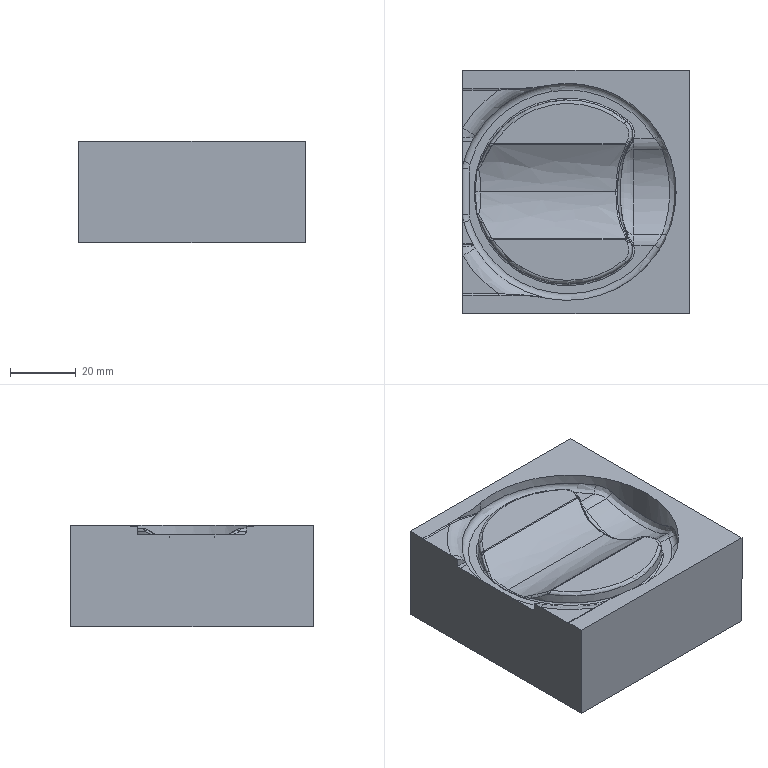NC program | NX | posted with a generic post | part box 69 x 74 x 31.001 mm
Lines 1117 to 2149 of 31411:
(CAVITY_MILL_COPY , TOOL : D4)
N2226 M6
N2228 G54
N2230 G17 G0 G90 X12.673 Y10.046 S3000 M3
N2232 G43 Z10.005 H0
N2234 Z-0.1
N2236 G94 G1 Z-0.3 F2500.
N2238 G3 X14.068 Y7.916 R3.
N2240 X14.297 Y7.776 R34.167
N2242 G1 X14.533 Y7.757
N2244 G3 X16.94 Y8.666 R3.
N2246 G1 Z-0.1
N2248 G0 Z0.305
N2250 X13.649 Y9.969
N2252 Z-0.25
N2254 G1 Z-0.45
N2256 G3 X15.101 Y7.876 R3.
N2258 X15.295 Y7.764 R33.672
N2260 G1 X15.409 Y7.743
N2262 X15.577 Y7.727
N2264 G3 X18.022 Y8.642 R3.
N2266 G1 Z-0.25
N2268 G0 Z0.
N2270 X14.426 Y9.899
N2272 Z-0.4
N2274 G1 Z-0.6
N2276 G3 X15.924 Y7.837 R3.
N2278 X16.12 Y7.73 R33.301
N2280 G1 X16.391 Y7.701
N2282 G3 X18.87 Y8.607 R3.
N2284 G1 Z-0.4
N2286 G0 Z-0.15
N2288 X15.106 Y9.829
N2290 Z-0.55
N2292 G1 Z-0.75
N2294 G3 X16.645 Y7.796 R3.
N2296 X16.893 Y7.667 R32.995
N2298 G2 X17.146 Y7.663 R52.17
N2300 G3 X19.356 Y8.582 R3.
N2302 G1 Z-0.55
N2304 G0 Z-0.3
N2306 X15.696 Y9.761
N2308 Z-0.7
N2310 G1 Z-0.9
N2312 G3 X17.27 Y7.755 R3.
N2314 X17.466 Y7.657 R32.745
N2316 G1 X17.665 Y7.652
N2318 G3 X19.884 Y8.549 R3.
N2320 G1 Z-0.7
N2322 G0 Z-0.45
N2324 X56.115 Y21.542
N2326 Z-0.843
N2328 G1 Z-1.043
N2330 G2 X55.66 Y20.526 R3.
N2332 X55.17 Y19.845 R28.83
N2334 G3 X55.097 Y20.583 R8.748
N2336 G2 X52.634 Y22.024 R4.06
N2338 X50.826 Y14.231 R6.748
N2340 X7.028 Y21.211 R29.544
N2342 X6.896 Y23.518 R2.382
N2344 G3 X7.155 Y25.291 R3.
N2346 G1 Z-0.843
N2348 G0 Z-0.6
N2350 X1.561 Y23.669
N2352 Z-0.843
N2354 G1 Z-1.043
N2356 G3 X2.694 Y22.308 R3.
N2358 G2 X3.485 Y21.41 R2.232
N2360 G1 X3.62 Y21.132
N2362 X4.229 Y20.072
N2364 X4.307 Y19.966
N2366 G3 X18.032 Y7.641 R32.512
N2368 G2 X26.165 Y6.727 R52.17
N2370 G3 X58.978 Y22.077 R30.83
N2372 X59.144 Y24.629 R3.
N2374 G1 Z-0.843
N2376 G0 Z-0.6
N2378 X56.27 Y21.786
N2380 Z-0.986
N2382 G1 Z-1.186
N2384 G2 X55.824 Y20.765 R3.
N2386 X55.358 Y20.101 R28.83
N2388 G3 X55.255 Y20.817 R9.856
N2390 G2 X52.692 Y22.346 R4.06
N2392 X53.392 Y19.644 R7.856
N2394 X50.952 Y14.079 R6.963
N2396 X6.729 Y21.317 R29.742
N2398 X6.627 Y23.748 R2.478
N2400 G3 X6.924 Y25.53 R3.
N2402 G1 Z-0.986
N2404 G0 Z-0.743
N2406 X1.486 Y23.67
N2408 Z-0.986
N2410 G1 Z-1.186
N2412 G3 X2.739 Y22.408 R3.
N2414 G2 X3.648 Y21.518 R2.244
N2416 G1 X4.372 Y20.219
N2418 X4.399 Y20.195
N2420 G3 X18.542 Y7.621 R32.314
N2422 G2 X26.165 Y6.727 R52.17
N2424 G3 X59.126 Y22.349 R30.83
N2426 X59.267 Y24.902 R3.
N2428 G1 Z-0.986
N2430 G0 Z-0.743
N2432 X56.359 Y21.93
N2434 Z-1.129
N2436 G1 Z-1.329
N2438 G2 X55.92 Y20.907 R3.
N2440 X55.474 Y20.262 R28.83
N2442 G3 X55.372 Y20.952 R8.855
N2444 G2 X52.734 Y22.527 R4.06
N2446 X52.97 Y22.01 R11.963
N2448 X51.542 Y14.485 R6.855
N2450 G1 X51.151 Y14.09
N2452 X51.036 Y13.977
N2454 G2 X6.622 Y21.239 R29.873
N2456 X6.418 Y23.934 R2.801
N2458 G3 X6.634 Y25.748 R3.
N2460 G1 Z-1.129
N2462 G0 Z-0.886
N2464 X1.458 Y23.67
N2466 Z-1.129
N2468 G1 Z-1.329
N2470 G3 X2.807 Y22.478 R3.
N2472 G2 X3.889 Y21.443 R2.217
N2474 G1 X4.044 Y21.132
N2476 X4.553 Y20.289
N2478 G3 X19.033 Y7.598 R32.134
N2480 G2 X26.165 Y6.727 R52.17
N2482 G3 X59.213 Y22.51 R30.83
N2484 X59.338 Y25.064 R3.
N2486 G1 Z-1.129
N2488 G0 Z-0.886
N2490 X56.416 Y22.021
N2492 Z-1.271
N2494 G1 Z-1.471
N2496 G2 X55.98 Y20.996 R3.
N2498 X55.558 Y20.382 R28.83
N2500 G3 X55.456 Y21.036 R8.975
N2502 G2 X52.828 Y22.553 R4.06
N2504 G1 X52.907 Y22.394
N2506 G2 X52.371 Y15.334 R6.975
N2508 G1 X52.354 Y15.309
N2510 G2 X51.095 Y13.905 R7.465
N2512 X6.471 Y21.307 R29.967
N2514 X6.266 Y24.16 R2.99
N2516 G3 X6.48 Y25.976 R3.
N2518 G1 Z-1.271
N2520 G0 Z-1.029
N2522 X1.227 Y23.67
N2524 Z-1.271
N2526 G1 Z-1.471
N2528 G3 X2.752 Y22.565 R3.
N2530 G2 X3.966 Y21.628 R2.24
N2532 G1 X4.659 Y20.398
N2534 X4.693 Y20.374
N2536 G3 X19.511 Y7.571 R31.97
N2538 G2 X26.165 Y6.727 R52.17
N2540 G3 X59.267 Y22.612 R30.83
N2542 X59.382 Y25.166 R3.
N2544 G1 Z-1.271
N2546 G0 Z-1.029
N2548 X56.469 Y22.109
N2550 Z-1.414
N2552 G1 Z-1.614
N2554 G2 X56.038 Y21.083 R3.
N2556 X55.618 Y20.466 R28.83
N2558 G3 X55.51 Y21.121 R9.082
N2560 G2 X52.85 Y22.667 R4.06
N2562 G1 X52.875 Y22.619
N2564 G2 X51.363 Y14.071 R7.082
N2566 G1 X51.169 Y13.892
N2568 X51.137 Y13.855
N2570 G2 X6.35 Y21.379 R30.032
N2572 X5.996 Y24.107 R3.403
N2574 G1 X6.035 Y24.226
N2576 G3 X6.115 Y26.019 R3.
N2578 G1 Z-1.414
N2580 G0 Z-1.171
N2582 X1.232 Y23.67
N2584 Z-1.414
N2586 G1 Z-1.614
N2588 G3 X2.833 Y22.592 R3.
N2590 G2 X4.134 Y21.628 R2.222
N2592 G1 X4.706 Y20.636
N2594 X4.823 Y20.453
N2596 G3 X19.979 Y7.54 R31.819
N2598 G2 X26.165 Y6.727 R52.17
N2600 G3 X59.318 Y22.71 R30.83
N2602 X59.425 Y25.265 R3.
N2604 G1 Z-1.414
N2606 G0 Z-1.171
N2608 X56.494 Y22.15
N2610 Z-1.557
N2612 G1 Z-1.757
N2614 G2 X56.064 Y21.123 R3.
N2616 X55.655 Y20.52 R28.83
N2618 G3 X55.548 Y21.159 R9.113
N2620 G2 X52.897 Y22.672 R4.06
N2622 G1 X52.924 Y22.619
N2624 G2 X51.858 Y14.509 R7.113
N2626 G1 X51.164 Y13.822
N2628 G2 X6.252 Y21.458 R30.075
N2630 X5.731 Y23.798 R3.914
N2632 X5.845 Y24.343 R2.473
N2634 G3 X5.866 Y26.148 R3.
N2636 G1 Z-1.557
N2638 G0 Z-1.314
N2640 X1.143 Y23.67
N2642 Z-1.557
N2644 G1 Z-1.757
N2646 G3 X2.865 Y22.624 R3.
N2648 G2 X4.302 Y21.628 R2.234
N2650 G1 X4.872 Y20.636
N2652 X4.942 Y20.525
N2654 G3 X20.442 Y7.505 R31.679
N2656 G2 X26.165 Y6.727 R52.17
N2658 G3 X59.342 Y22.756 R30.83
N2660 X59.444 Y25.311 R3.
N2662 G1 Z-1.557
N2664 G0 Z-1.314
N2666 X56.503 Y22.164
N2668 Z-1.7
N2670 G1 Z-1.9
N2672 G2 X56.073 Y21.136 R3.
N2674 X55.676 Y20.549 R28.83
N2676 G3 X55.57 Y21.17 R9.175
N2678 G2 X52.954 Y22.623 R4.06
N2680 G1 X52.984 Y22.563
N2682 G2 X51.385 Y13.991 R7.175
N2684 G1 X51.363 Y13.982
N2686 X51.193 Y13.838
N2688 X51.179 Y13.804
N2690 G2 X6.174 Y21.544 R30.097
N2692 X5.609 Y24.134 R4.083
N2694 X5.686 Y24.517 R2.426
N2696 G3 X5.637 Y26.315 R3.
N2698 G1 Z-1.7
N2700 G0 Z-1.457
N2702 X0.932 Y23.67
N2704 Z-1.7
N2706 G1 Z-1.9
N2708 G3 X2.842 Y22.654 R3.
N2710 G2 X4.448 Y21.628 R2.194
N2712 G1 X5.02 Y20.636
N2714 X5.052 Y20.593
N2716 G3 X20.905 Y7.466 R31.55
N2718 G2 X26.165 Y6.727 R52.17
N2720 G3 X59.35 Y22.771 R30.83
N2722 X59.451 Y25.326 R3.
N2724 G1 Z-1.7
N2726 G0 Z-1.457
N2728 X56.511 Y22.177
N2730 Z-1.843
N2732 G1 Z-2.043
N2734 G2 X56.082 Y21.15 R3.
N2736 X55.693 Y20.575 R28.83
N2738 G3 X55.588 Y21.182 R9.162
N2740 G2 X52.975 Y22.618 R4.06
N2742 X51.402 Y13.991 R7.162
N2744 G1 X51.363 Y13.969
N2746 X51.202 Y13.832
N2748 X51.189 Y13.802
N2750 G2 X6.041 Y21.753 R30.106
N2752 X5.439 Y24.142 R4.341
N2754 X5.518 Y24.669 R2.475
N2756 G3 X5.429 Y26.472 R3.
N2758 G1 Z-1.843
N2760 G0 Z-1.6
N2762 X0.586 Y23.707
N2764 Z-1.843
N2766 G1 Z-2.043
N2768 G3 X2.705 Y22.694 R3.
N2770 G1 X2.821 Y22.689
N2772 G2 X4.583 Y21.628 R2.17
N2774 G1 X5.155 Y20.655
N2776 G3 X21.371 Y7.422 R31.43
N2778 G2 X26.165 Y6.727 R52.17
N2780 G3 X59.358 Y22.786 R30.83
N2782 X59.457 Y25.341 R3.
N2784 G1 Z-1.843
N2786 G0 Z-1.6
N2788 X56.524 Y22.199
N2790 Z-1.986
N2792 G1 Z-2.186
N2794 G2 X56.096 Y21.171 R3.
N2796 X55.702 Y20.587 R28.83
N2798 G3 X55.594 Y21.204 R9.177
N2800 G2 X52.961 Y22.669 R4.06
N2802 X51.2 Y13.801 R7.177
N2804 X5.881 Y22.013 R30.113
N2806 X5.298 Y24.401 R4.38
N2808 X5.372 Y24.878 R2.493
N2810 G3 X5.274 Y26.684 R3.
N2812 G1 Z-1.986
N2814 G0 Z-1.743
N2816 X0.31 Y23.748
N2818 Z-1.986
N2820 G1 Z-2.186
N2822 G3 X2.461 Y22.749 R3.
N2824 G1 X2.821 Y22.739
N2826 G2 X4.712 Y21.628 R2.155
N2828 G1 X5.25 Y20.713
N2830 G3 X21.846 Y7.374 R31.318
N2832 G2 X26.165 Y6.727 R52.17
N2834 G3 X59.37 Y22.81 R30.83
N2836 X59.467 Y25.365 R3.
N2838 G1 Z-1.986
N2840 G0 Z-1.743
N2842 X56.53 Y22.209
N2844 Z-2.129
N2846 G1 Z-2.329
N2848 G2 X56.102 Y21.181 R3.
N2850 X55.71 Y20.598 R28.83
N2852 G3 X55.601 Y21.214 R9.178
N2854 G2 X52.961 Y22.685 R4.06
N2856 X51.211 Y13.801 R7.178
N2858 X5.725 Y22.273 R30.121
N2860 X5.165 Y24.603 R4.339
N2862 X5.221 Y25.026 R2.495
N2864 G3 X5.057 Y26.827 R3.
N2866 G1 Z-2.129
N2868 G0 Z-1.886
N2870 X0.015 Y23.799
N2872 Z-2.129
N2874 G1 Z-2.329
N2876 G3 X2.254 Y22.806 R3.
N2878 G1 X2.821 Y22.807
N2880 G2 X4.802 Y21.681 R2.188
N2882 G1 X5.338 Y20.767
N2884 G3 X22.337 Y7.319 R31.215
N2886 G2 X26.165 Y6.727 R52.17
N2888 G3 X59.376 Y22.822 R30.83
N2890 X59.472 Y25.377 R3.
N2892 G1 Z-2.129
N2894 G0 Z-1.886
N2896 X56.536 Y22.22
N2898 Z-2.271
N2900 G1 Z-2.471
N2902 G2 X56.109 Y21.191 R3.
N2904 X55.717 Y20.609 R28.83
N2906 G3 X55.608 Y21.224 R9.17
N2908 G2 X52.95 Y22.716 R4.06
N2910 G1 X53.002 Y22.619
N2912 G2 X51.222 Y13.801 R7.17
N2914 X5.573 Y22.533 R30.128
N2916 X5.103 Y25.204 R3.856
N2918 G3 X4.886 Y26.997 R3.
N2920 G1 Z-2.271
N2922 G0 Z-2.029
N2924 X-0.118 Y23.875
N2926 Z-2.271
N2928 G1 Z-2.471
N2930 G3 X2.114 Y22.883 R3.
N2932 G1 X2.995 Y22.884
N2934 G2 X4.778 Y21.879 R2.082
N2936 G1 X5.421 Y20.817
N2938 G3 X22.855 Y7.255 R31.119
N2940 G2 X26.165 Y6.727 R52.17
N2942 G3 X59.382 Y22.833 R30.83
N2944 X59.477 Y25.389 R3.
N2946 G1 Z-2.271
N2948 G0 Z-2.029
N2950 X56.536 Y22.219
N2952 Z-2.414
N2954 G1 Z-2.614
N2956 G2 X56.109 Y21.191 R3.
N2958 X55.726 Y20.621 R28.83
N2960 G3 X55.619 Y21.222 R9.177
N2962 G2 X52.988 Y22.669 R4.06
N2964 X51.234 Y13.8 R7.177
N2966 X5.424 Y22.792 R30.136
N2968 X4.925 Y25.175 R4.302
N2970 G1 X4.948 Y25.364
N2972 G3 X4.681 Y27.151 R3.
N2974 G1 Z-2.414
N2976 G0 Z-2.171
N2978 X-0.227 Y23.972
N2980 Z-2.414
N2982 G1 Z-2.614
N2984 G3 X2.001 Y22.989 R3.
N2986 G1 X3.011 Y22.991
N2988 G2 X4.887 Y21.886 R2.136
N2990 G1 X5.029 Y21.628
N2992 X5.497 Y20.863
N2994 G3 X23.421 Y7.181 R31.029
N2996 G2 X26.165 Y6.727 R52.17
N2998 G3 X59.382 Y22.833 R30.83
N3000 X59.477 Y25.388 R3.
N3002 G1 Z-2.414
N3004 G0 Z-2.171
N3006 X56.541 Y22.228
N3008 Z-2.557
N3010 G1 Z-2.757
N3012 G2 X56.114 Y21.199 R3.
N3014 X55.734 Y20.633 R28.83
N3016 G3 X55.627 Y21.23 R9.176
N3018 G2 X52.993 Y22.675 R4.06
N3020 X51.245 Y13.8 R7.176
N3022 X5.278 Y23.052 R30.143
N3024 X4.802 Y25.49 R4.339
N3026 G1 X4.815 Y25.586
N3028 G3 X4.537 Y27.371 R3.
N3030 G1 Z-2.557
N3032 G0 Z-2.314
N3034 X-0.448 Y24.062
N3036 Z-2.557
N3038 G1 Z-2.757
N3040 G3 X1.762 Y23.096 R3.
N3042 G1 X3.053 Y23.099
N3044 G2 X4.892 Y22.052 R2.13
N3046 G1 X5.568 Y20.907
N3048 G3 X24.074 Y7.086 R30.946
N3050 G2 X26.165 Y6.727 R52.17
N3052 G3 X59.387 Y22.842 R30.83
N3054 X59.481 Y25.398 R3.
N3056 G1 Z-2.557
N3058 G0 Z-2.314
N3060 X56.546 Y22.235
N3062 Z-2.7
N3064 G1 Z-2.9
N3066 G2 X56.119 Y21.207 R3.
N3068 X55.739 Y20.64 R28.83
N3070 G3 X55.63 Y21.237 R9.142
N3072 G2 X52.967 Y22.72 R4.06
N3074 X53.061 Y22.536 R25.392
N3076 X51.258 Y13.801 R7.142
N3078 X5.143 Y23.299 R30.15
N3080 X4.675 Y25.638 R4.396
N3082 G1 X4.682 Y25.71
N3084 G3 X4.325 Y27.48 R3.
N3086 G1 Z-2.7
N3088 G0 Z-2.457
N3090 X-0.189 Y24.241
N3092 Z-2.7
N3094 G1 Z-2.9
N3096 G3 X1.9 Y23.331 R3.
N3098 G2 X3.35 Y23.232 R15.61
N3100 X4.883 Y22.226 R2.04
N3102 G1 X5.515 Y21.132
N3104 X5.63 Y20.945
N3106 G3 X24.898 Y6.955 R30.873
N3108 G2 X26.165 Y6.727 R52.17
N3110 G3 X59.392 Y22.851 R30.83
N3112 X59.485 Y25.407 R3.
N3114 G1 Z-2.7
N3116 G0 Z-2.457
N3118 X56.551 Y22.244
N3120 Z-2.843
N3122 G1 Z-3.043
N3124 G2 X56.124 Y21.215 R3.
N3126 X55.748 Y20.655 R28.83
N3128 G3 X55.639 Y21.245 R9.141
N3130 G2 X52.977 Y22.721 R4.06
N3132 G1 X53.032 Y22.619
N3134 X53.117 Y22.446
N3136 G2 X51.272 Y13.803 R7.141
N3138 X4.997 Y23.571 R30.158
N3140 X4.638 Y26.306 R3.927
N3142 X6.296 Y28.078 R2.426
N3144 G3 X7.849 Y29.183 R3.
N3146 G1 Z-2.843
N3148 G0 Z-2.6
N3150 X3.17 Y33.68
N3152 Z-2.843
N3154 G1 Z-3.043
N3156 G3 X2.17 Y31.444 R3.
N3158 G1 Y29.189
N3160 X2.195 Y29.214
N3162 X2.228 Y29.2
N3164 Y29.165
N3166 X2.403 Y28.368
N3168 G3 X58.256 Y20.842 R30.83
N3170 G1 X58.683 Y21.557
N3172 G3 X59.397 Y22.861 R30.83
N3174 X59.489 Y25.416 R3.
N3176 G1 Z-2.843
N3178 G0 Z-2.6
N3180 X56.545 Y22.251
N3182 Z-2.986
N3184 G1 Z-3.186
N3186 G2 X56.119 Y21.224 R3.
N3188 X55.753 Y20.677 R28.821
N3190 G3 X55.646 Y21.253 R9.134
N3192 G2 X52.974 Y22.738 R4.06
N3194 X53.076 Y22.54 R28.8
N3196 X51.286 Y13.805 R7.134
N3198 X4.861 Y23.831 R30.166
N3200 X4.525 Y26.586 R4.104
N3202 X6.205 Y28.343 R2.403
N3204 G3 X7.787 Y29.434 R3.
N3206 G1 Z-2.986
N3208 G0 Z-2.743
N3210 X3.179 Y33.944
N3212 Z-2.986
N3214 G1 Z-3.186
N3216 G3 X2.179 Y31.708 R3.
N3218 G1 Y30.
N3220 G3 X2.412 Y28.37 R5.821
N3222 X58.249 Y20.846 R30.821
N3224 G1 X59.232 Y22.547
N3226 G3 X59.401 Y22.87 R30.83
N3228 X59.493 Y25.426 R3.
N3230 G1 Z-2.986
N3232 G0 Z-2.743
N3234 X56.527 Y22.256
N3236 Z-3.129
N3238 G1 Z-3.329
N3240 G2 X56.102 Y21.232 R3.
N3242 X55.756 Y20.716 R28.801
N3244 G3 X55.653 Y21.261 R9.133
N3246 G2 X52.977 Y22.747 R4.06
N3248 X53.082 Y22.545 R30.654
N3250 X51.298 Y13.805 R7.133
N3252 X4.727 Y24.093 R30.173
N3254 X4.307 Y26.398 R4.614
N3256 X6.142 Y28.613 R2.496
N3258 G3 X7.749 Y29.7 R3.
N3260 G1 Z-3.129
N3262 G0 Z-2.886
N3264 X3.199 Y34.213
N3266 Z-3.129
N3268 G1 Z-3.329
N3270 G3 X2.199 Y31.977 R3.
N3272 G1 Y30.
N3274 G3 X2.431 Y28.376 R5.801
N3276 X58.232 Y20.857 R30.801
N3278 G1 X59.381 Y22.846
N3280 G3 X59.538 Y25.534 R3.
N3282 G1 Z-3.129
N3284 G0 Z-2.886
N3286 X56.495 Y22.26
N3288 Z-3.271
N3290 G1 Z-3.471
N3292 G2 X56.07 Y21.241 R3.
N3294 X55.756 Y20.77 R28.771
N3296 G3 X55.659 Y21.269 R9.126
N3298 G2 X52.973 Y22.765 R4.06
N3300 X53.081 Y22.558 R49.362
N3302 X51.312 Y13.807 R7.126
N3304 X4.594 Y24.359 R30.181
N3306 X4.245 Y26.967 R4.318
N3308 X6.048 Y28.897 R2.429
N3310 G3 X7.692 Y29.969 R3.
N3312 G1 Z-3.271
N3314 G0 Z-3.029
N3316 X3.229 Y34.494
N3318 Z-3.271
N3320 G1 Z-3.471
N3322 G3 X2.229 Y32.258 R3.
N3324 G1 Y30.
N3326 G3 X2.46 Y28.384 R5.771
N3328 X58.206 Y20.873 R30.771
N3330 X59.288 Y22.73 R65.68
N3332 X59.451 Y25.326 R3.
N3334 G1 Z-3.271
N3336 G0 Z-3.029
N3338 X56.455 Y22.272
N3340 Z-3.414
N3342 G1 Z-3.614
N3344 G2 X56.031 Y21.258 R3.
N3346 X55.754 Y20.843 R28.728
N3348 G3 X55.666 Y21.285 R9.146
N3350 G2 X52.972 Y22.781 R4.06
N3352 G1 X53.064 Y22.619
N3354 G2 X51.312 Y13.798 R7.146
N3356 X4.461 Y24.634 R30.188
N3358 X4.215 Y27.578 R4.217
N3360 X5.983 Y29.193 R2.35
N3362 G3 X7.707 Y30.249 R3.
N3364 G1 Z-3.414
N3366 G0 Z-3.171
N3368 X3.272 Y34.783
N3370 Z-3.414
N3372 G1 Z-3.614
N3374 G3 X2.272 Y32.547 R3.
N3376 G1 Y30.
N3378 G3 X2.501 Y28.396 R5.728
N3380 X58.169 Y20.895 R30.728
N3382 X59.253 Y22.706 R63.482
N3384 X59.443 Y25.307 R3.
N3386 G1 Z-3.414
N3388 G0 Z-3.171
N3390 X56.402 Y22.288
N3392 Z-3.557
N3394 G1 Z-3.757
N3396 G2 X55.979 Y21.28 R3.
N3398 X55.75 Y20.936 R28.673
N3400 G3 X55.674 Y21.304 R9.122
N3402 G2 X52.973 Y22.798 R4.06
N3404 G1 X52.985 Y22.776
N3406 G2 X51.342 Y13.812 R7.122
N3408 X4.33 Y24.912 R30.196
N3410 X4.021 Y27.578 R4.353
N3412 X5.936 Y29.493 R2.384
N3414 G3 X7.706 Y30.531 R3.
N3416 G1 Z-3.557
N3418 G0 Z-3.314
N3420 X3.327 Y35.075
N3422 Z-3.557
N3424 G1 Z-3.757
N3426 G3 X2.327 Y32.839 R3.
N3428 G1 Y30.
N3430 G3 X2.554 Y28.412 R5.673
N3432 X58.032 Y20.779 R30.673
N3434 G1 X58.107 Y20.926
N3436 X59.174 Y22.619
N3438 X59.204 Y22.673
N3440 G3 X59.402 Y25.211 R3.
N3442 G1 Z-3.557
N3444 G0 Z-3.314
N3446 X56.344 Y22.323
N3448 Z-3.7
N3450 G1 Z-3.9
N3452 G2 X55.923 Y21.321 R3.
N3454 X55.74 Y21.045 R28.603
N3456 G3 X55.676 Y21.341 R9.12
N3458 G2 X52.963 Y22.832 R4.06
N3460 G1 X52.991 Y22.782
N3462 G2 X51.355 Y13.814 R7.12
N3464 X4.199 Y25.197 R30.203
N3466 X3.952 Y28.074 R4.251
N3468 X5.883 Y29.808 R2.39
N3470 G3 X7.706 Y30.837 R3.
N3472 G1 Z-3.7
N3474 G0 Z-3.457
N3476 X3.397 Y35.376
N3478 Z-3.7
N3480 G1 Z-3.9
N3482 G3 X2.397 Y33.14 R3.
N3484 G1 Y30.
N3486 G3 X2.621 Y28.431 R5.603
N3488 X58.063 Y20.96 R30.603
N3490 G1 X58.143 Y21.132
N3492 X59.109 Y22.609
N3494 X59.134 Y22.647
N3496 G3 X59.44 Y25.301 R3.
N3498 G1 Z-3.7
N3500 G0 Z-3.457
N3502 X56.277 Y22.373
N3504 Z-3.843
N3506 G1 Z-4.043
N3508 G2 X55.857 Y21.376 R3.
N3510 X55.723 Y21.173 R28.518
N3512 G3 X55.674 Y21.391 R9.117
N3514 G2 X52.939 Y22.889 R4.06
N3516 G1 X52.985 Y22.807
N3518 G2 X51.368 Y13.815 R7.117
N3520 X4.066 Y25.495 R30.211
N3522 X3.751 Y28.107 R4.801
N3524 X5.923 Y30.139 R2.423
N3526 G3 X7.907 Y31.152 R3.
N3528 G1 Z-3.843
N3530 G0 Z-3.6
N3532 X3.482 Y35.701
N3534 Z-3.843
N3536 G1 Z-4.043
N3538 G3 X2.482 Y33.465 R3.
N3540 G1 Y30.
N3542 G3 X2.703 Y28.455 R5.518
N3544 X58.215 Y21.375 R30.518
N3546 G2 X58.966 Y22.516 R15.261
N3548 G1 X59.046 Y22.627
N3550 G3 X59.446 Y25.316 R3.
N3552 G1 Z-3.843
N3554 G0 Z-3.6
N3556 X56.198 Y22.439
N3558 Z-3.986
N3560 G1 Z-4.186
N3562 G2 X55.781 Y21.448 R3.
N3564 G1 X55.7 Y21.325
N3566 X55.668 Y21.457
N3568 G2 X52.898 Y22.972 R4.06
N3570 G1 X52.975 Y22.838
N3572 G2 X51.386 Y13.82 R7.108
N3574 X3.934 Y25.802 R30.218
N3576 X3.598 Y28.335 R5.386
N3578 X5.923 Y30.472 R2.395
N3580 G3 X8.09 Y31.473 R3.
N3582 G1 Z-3.986
N3584 G0 Z-3.743
N3586 X3.585 Y36.018
N3588 Z-3.986
N3590 G1 Z-4.186
N3592 G3 X2.585 Y33.782 R3.
N3594 G1 Y30.
N3596 G3 X2.802 Y28.484 R5.415
N3598 X57.903 Y21.059 R30.415
N3600 G2 X58.908 Y22.586 R21.391
N3602 G3 X59.368 Y25.135 R3.
N3604 G1 Z-3.986
N3606 G0 Z-3.743
N3608 X56.097 Y22.511
N3610 Z-4.129
N3612 G1 Z-4.329
N3614 G2 X55.681 Y21.527 R3.
N3616 G1 X55.664 Y21.5
N3618 X55.657 Y21.529
N3620 G2 X52.867 Y23.044 R4.06
N3622 G3 X52.968 Y22.869 R23.759
N3624 G2 X51.382 Y13.807 R7.129
N3626 X3.8 Y26.121 R30.226
N3628 X3.42 Y28.57 R5.796
N3630 X5.793 Y30.82 R2.39
N3632 G1 X6.013
N3634 G3 X8.248 Y31.821 R3.
N3636 G1 Z-4.129
N3638 G0 Z-3.886
N3640 X3.712 Y36.36
N3642 Z-4.129
N3644 G1 Z-4.329
N3646 G3 X2.712 Y34.124 R3.
N3648 G1 Y30.
N3650 G3 X2.923 Y28.519 R5.288
N3652 X57.818 Y21.164 R30.288
N3654 G2 X58.749 Y22.542 R19.151
N3656 G3 X59.265 Y24.982 R3.
N3658 G1 Z-4.129
N3660 G0 Z-2.029
N3662 X3.868 Y36.723
N3664 Z-4.271
N3666 G1 Z-4.471
N3668 G3 X2.868 Y34.487 R3.
N3670 G1 Y30.
N3672 G3 X3.073 Y28.563 R5.132
N3674 X3.272 Y27.909 R30.132
N3676 G2 X3.889 Y30.45 R2.841
N3678 X5.493 Y31.18 R2.127
N3680 G1 X6.189
N3682 G3 X8.425 Y32.18 R3.
N3684 G1 Z-4.271
N3686 G0 Z-4.029
N3688 X4.068 Y37.103
N3690 Z-4.414
N3692 G1 Z-4.614
N3694 G3 X3.068 Y34.867 R3.
N3696 G1 Y30.
N3698 X3.072 Y29.802
N3700 G2 X5.298 Y31.557 R2.332
N3702 G1 X6.385 Y31.56
N3704 G3 X8.618 Y32.567 R3.
N3706 G1 Z-4.414
N3708 G0 Z-4.171
N3710 X4.347 Y37.507
N3712 Z-4.557
N3714 G1 Z-4.757
N3716 G3 X3.347 Y35.27 R3.
N3718 G1 Y31.228
N3720 G2 X4.951 Y31.946 R2.152
N3722 G1 X6.77 Y31.947
N3724 G3 X9.006 Y32.948 R3.
N3726 G1 Z-4.557
N3728 G0 Z-4.314
N3730 X4.901 Y37.918
N3732 Z-4.7
N3734 G1 Z-4.9
N3736 G3 X3.901 Y35.681 R3.
N3738 G1 Y32.439
N3740 X3.939 Y32.408
N3742 X7.054 Y32.406
N3744 G3 X9.291 Y33.405 R3.
N3746 G1 Z-4.7
N3748 G0 Z-4.457
N3750 X7.344 Y38.73
N3752 Z-4.849
N3754 G1 Z-5.049
N3756 G3 X5.963 Y36.1 R3.
N3758 X6.277 Y32.874 R26.052
N3760 G1 X9.264 Y32.876
N3762 G3 X11.499 Y33.877 R3.
N3764 G1 Z-4.849
N3766 G0 Z10.005
N3768 X52.638 Y25.747
N3770 Z-4.271
N3772 G1 Z-4.471
N3774 G3 X52.816 Y23.15 R3.
N3776 X52.98 Y22.866 R22.364
N3778 G2 X52.354 Y14.781 R7.086
N3780 G3 X57.648 Y21.186 R30.132
N3782 G1 X57.921 Y21.628
N3784 X58.711 Y22.651
N3786 G3 X59.279 Y25.058 R3.
N3788 G1 Z-4.271
N3790 G0 Z-4.029
N3792 X52.585 Y25.876
N3794 Z-4.414
N3796 G1 Z-4.614
N3798 G3 X52.751 Y23.287 R3.
N3800 X53.141 Y22.619 R23.55
N3802 G2 X52.998 Y15.669 R7.103
N3804 G3 X57.478 Y21.29 R29.932
N3806 G2 X58.394 Y22.576 R12.08
N3808 G3 X59.052 Y24.808 R3.
N3810 G1 Z-4.414
N3812 G0 Z-4.171
N3814 X52.521 Y26.081
N3816 Z-4.557
N3818 G1 Z-4.757
N3820 G3 X52.681 Y23.452 R3.
N3822 X53.344 Y22.355 R22.236
N3824 G2 X53.549 Y16.63 R7.044
N3826 G3 X57.254 Y21.459 R29.653
N3828 G2 X58.172 Y22.664 R9.395
N3830 G3 X58.937 Y24.802 R3.
N3832 G1 Z-4.557
N3834 G0 Z-4.314
N3836 X52.375 Y26.47
N3838 Z-4.7
N3840 G1 Z-4.9
N3842 G3 X52.547 Y23.721 R3.
N3844 X52.849 Y23.244 R11.632
N3846 G1 X52.943 Y23.115
N3848 X53.32 Y22.619
N3850 G2 X54.238 Y18.232 R5.564
N3852 G3 X56.479 Y21.267 R29.099
N3854 G1 X56.493 Y21.314
N3856 G2 X57.464 Y22.566 R2.2
N3858 G3 X58.91 Y24.953 R3.
N3860 G1 Z-4.7
N3862 G0 Z-4.457
N3864 X51.615 Y28.465
N3866 Z-4.849
N3868 G1 Z-5.049
N3870 G3 X51.487 Y26.001 R3.
N3872 X52.368 Y24.045 R20.855
N3874 G1 X54.299
N3876 G3 X56.535 Y25.045 R3.
N3878 G1 Z-4.849
N3880 G0 Z-4.6
N3882 X51.457 Y28.975
N3884 Z-4.998
N3886 G1 Z-5.198
N3888 G3 X51.294 Y26.543 R3.
N3890 G1 X51.363 Y26.356
N3892 G3 X52.129 Y24.539 R20.662
N3894 G1 X54.134
N3896 G3 X56.371 Y25.539 R3.
N3898 G1 Z-4.998
N3900 G0 Z-4.749
N3902 X51.342 Y29.404
N3904 Z-5.146
N3906 G1 Z-5.346
N3908 G3 X51.161 Y26.958 R3.
N3910 G1 X51.295 Y26.586
N3912 X51.858 Y25.145
N3914 X51.975 Y24.909
N3916 X54.026
N3918 G3 X56.262 Y25.909 R3.
N3920 G1 Z-5.146
N3922 G0 Z-4.898
N3924 X51.256 Y29.784
N3926 Z-5.295
N3928 G1 Z-5.495
N3930 G3 X51.044 Y27.331 R3.
N3932 X51.482 Y26.091 R244.214
N3934 G1 X51.848 Y25.187
N3936 X52. Y25.213
N3938 X53.975
N3940 G3 X56.211 Y26.213 R3.
N3942 G1 Z-5.295
N3944 G0 Z-5.046
N3946 X51.173 Y30.18
N3948 Z-5.444
N3950 G1 Z-5.644
N3952 G3 X50.936 Y27.742 R3.
N3954 G1 X51.49 Y26.091
N3956 X51.734 Y25.473
N3958 X51.982 Y25.442
N3960 X52. Y25.475
N3962 X53.912
N3964 G3 X56.148 Y26.475 R3.
N3966 G1 Z-5.444
N3968 G0 Z-5.195
N3970 X51.17 Y30.35
N3972 Z-5.593
N3974 G1 Z-5.793
N3976 G3 X50.899 Y27.877 R3.
N3978 X51.647 Y25.705 R83.909
N3980 G1 X53.829
N3982 G3 X56.065 Y26.705 R3.
N3984 G1 Z-5.593
N3986 G0 Z-5.344
N3988 X51.139 Y30.626
N3990 Z-5.742
N3992 G1 Z-5.942
N3994 G3 X50.829 Y28.152 R3.
N3996 X51.554 Y25.965 R72.711
N3998 G1 X51.994 Y25.887
N4000 X52. Y25.911
N4002 X53.793
N4004 G3 X56.029 Y26.911 R3.
N4006 G1 Z-5.742
N4008 G0 Z-5.493
N4010 X51.043 Y31.116
N4012 Z-5.891
N4014 G1 Z-6.091
N4016 G3 X50.692 Y28.674 R3.
N4018 X51.475 Y26.201 R51.124
N4020 G1 X52. Y26.097
N4022 X53.799
N4024 G3 X56.035 Y27.097 R3.
N4026 G1 Z-5.891
N4028 G0 Z-5.642
N4030 X51.106 Y31.112
N4032 Z-6.039
N4034 G1 Z-6.239
N4036 G3 X50.726 Y28.64 R3.
N4038 X51.395 Y26.443 R62.11
N4040 X52.063 Y26.273 R1.392
N4042 G1 X53.748
N4044 G3 X55.984 Y27.273 R3.
N4046 G1 Z-6.039
N4048 G0 Z-5.791
N4050 X51.093 Y31.349
N4052 Z-6.188
N4054 G1 Z-6.388
N4056 G3 X50.68 Y28.882 R3.
N4058 X51.318 Y26.686 R61.266
N4060 X52.055 Y26.452 R1.588
N4062 G1 X53.729
N4064 G3 X55.965 Y27.452 R3.
N4066 G1 Z-6.188
N4068 G0 Z-5.939
N4070 X51.085 Y31.609
N4072 Z-6.337
N4074 G1 Z-6.537
N4076 G3 X50.63 Y29.14 R3.
N4078 X51.242 Y26.937 R52.019
N4080 X52.081 Y26.636 R1.568
N4082 G1 X53.709
N4084 G3 X55.945 Y27.636 R3.
N4086 G1 Z-6.337
N4088 G0 Z-6.088
N4090 X51.087 Y31.846
N4092 Z-6.486
N4094 G1 Z-6.686
N4096 G3 X50.589 Y29.378 R3.
N4098 X51.171 Y27.193 R43.413
N4100 X52.094 Y26.824 R1.531
N4102 G1 X53.687
N4104 G3 X55.923 Y27.824 R3.
N4106 G1 Z-6.486
N4108 G0 Z-6.237
N4110 X51.089 Y32.
N4112 Z-6.635
N4114 G1 Z-6.835
N4116 G3 X50.562 Y29.582 R3.
N4118 X51.097 Y27.467 R29.566
N4120 X52.106 Y27.017 R1.517
N4122 G1 X53.665
N4124 G3 X55.901 Y28.017 R3.
N4126 G1 Z-6.635
N4128 G0 Z-6.386
N4130 X51.089 Y32.228
N4132 Z-6.784
N4134 G1 Z-6.984
N4136 G3 X50.532 Y29.809 R3.
N4138 X51.023 Y27.758 R30.203
N4140 X52.235 Y27.215 R1.625
N4142 G1 X53.645
N4144 G3 X55.881 Y28.215 R3.
N4146 G1 Z-6.784
N4148 G0 Z-6.535
N4150 X51.093 Y32.519
N4152 Z-6.932
N4154 G1 Z-7.132
N4156 G3 X50.494 Y30.066 R3.
N4158 X50.969 Y28.045 R29.169
N4160 X52. Y27.419 R1.766
N4162 G1 X53.655
N4164 G3 X55.891 Y28.419 R3.
N4166 G1 Z-6.932
N4168 G0 Z-6.684
N4170 X51.094 Y32.744
N4172 Z-7.081
N4174 G1 Z-7.281
N4176 G3 X50.471 Y30.286 R3.
N4178 X50.868 Y28.453 R37.929
N4180 X52.089 Y27.628 R1.632
N4182 G1 X53.608
N4184 G3 X55.844 Y28.628 R3.
N4186 G1 Z-7.081
N4188 G0 Z-6.832
N4190 X51.092 Y33.037
N4192 Z-7.23
N4194 G1 Z-7.43
N4196 G3 X50.429 Y30.589 R3.
N4198 X50.794 Y28.758 R37.484
N4200 X52.089 Y27.842 R1.836
N4202 G1 X53.595
N4204 G3 X55.831 Y28.842 R3.
N4206 G1 Z-7.23
N4208 G0 Z-6.981
N4210 X51.107 Y33.223
N4212 Z-7.379
N4214 G1 Z-7.579
N4216 G3 X50.42 Y30.793 R3.
N4218 X50.636 Y29.562 R42.587
N4220 X52.053 Y28.063 R1.828
N4222 G1 X53.58
N4224 G3 X55.816 Y29.063 R3.
N4226 G1 Z-7.379
N4228 G0 Z-7.13
N4230 X51.11 Y33.493
N4232 Z-7.528
N4234 G1 Z-7.728
N4236 G3 X50.389 Y31.068 R3.
N4238 X50.575 Y29.922 R40.741
N4240 X52.087 Y28.291 R2.051
N4242 G1 X53.565
N4244 G3 X55.801 Y29.291 R3.
N4246 G1 Z-7.528
N4248 G0 Z-7.279
N4250 X51.113 Y33.763
N4252 Z-7.677
N4254 G1 Z-7.877
N4256 G3 X50.363 Y31.351 R3.
N4258 X50.478 Y30.553 R42.445
N4260 X51.611 Y28.68 R2.712
N4262 G1 X52.122 Y28.525
N4264 X53.554
N4266 G3 X55.79 Y29.525 R3.
N4268 G1 Z-7.677
N4270 G0 Z-7.428
N4272 X51.119 Y34.019
N4274 Z-7.825
N4276 G1 Z-8.025
N4278 G3 X50.346 Y31.617 R3.
N4280 X50.42 Y31.049 R44.017
N4282 X51.457 Y29.057 R3.373
N4284 X52.19 Y28.767 R1.074